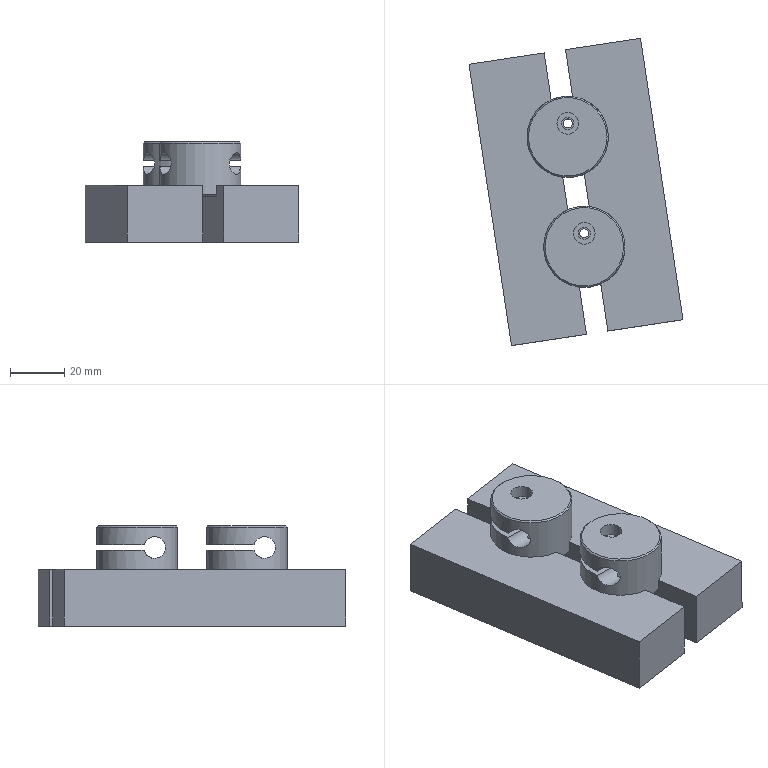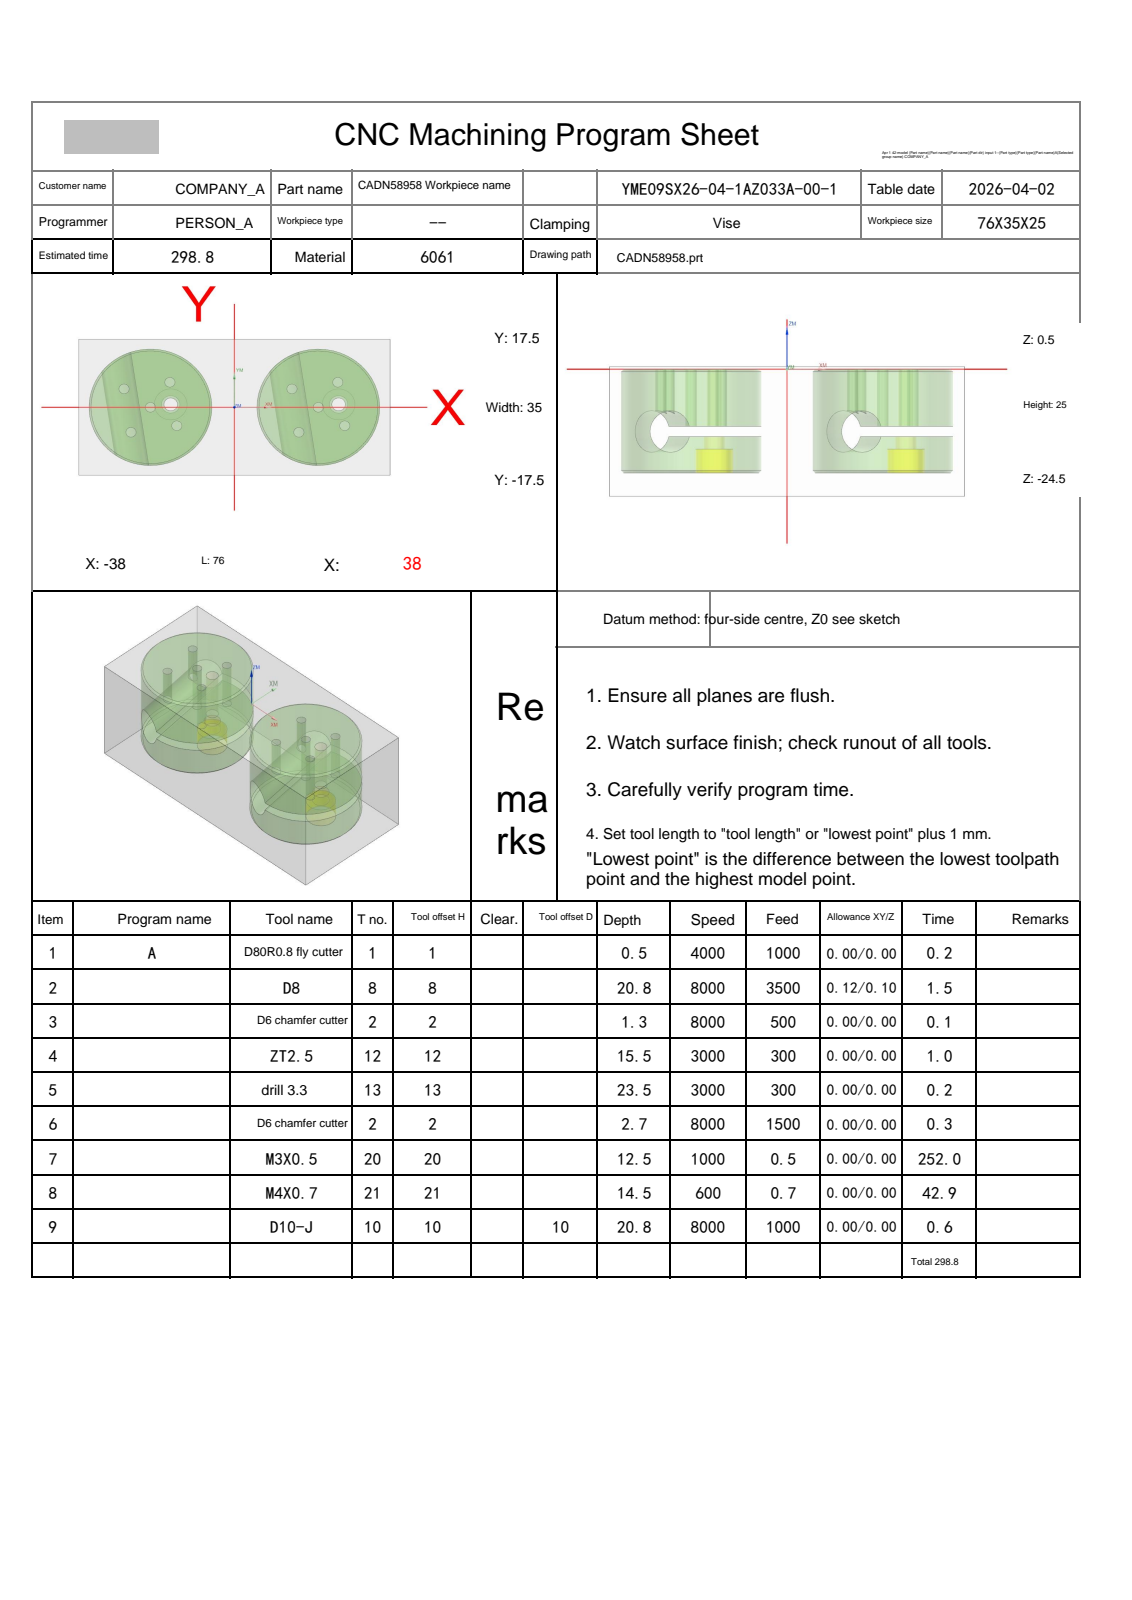NC program | NX | posted by the shop | part box 78.946 x 113.372 x 37 mm
Lines 35 to 955 of 2409:
N2 T08 M06
(D8  D=8. R=0. H=08 ce=0.12 di=0.10)
G00 G90 G54 X-19.131 Y27.067 M03 S8000
G43 H08 Z20.
M08
Z-8.15
G01 X-19.124 Y26.967 Z-8.775 F3500.
X-19.117 Y26.868 Z-9.022
X-19.11 Y26.768 Z-9.204
X-19.103 Y26.668 Z-9.35
X-19.096 Y26.568 Z-9.473
X-19.089 Y26.469 Z-9.578
X-19.082 Y26.369 Z-9.67
X-19.075 Y26.269 Z-9.75
X-19.068 Y26.169 Z-9.82
X-19.061 Y26.07 Z-9.882
X-19.054 Y25.97 Z-9.936
X-19.047 Y25.87 Z-9.983
X-19.04 Y25.77 Z-10.024
X-19.033 Y25.671 Z-10.058
X-19.026 Y25.571 Z-10.086
X-19.019 Y25.471 Z-10.11
X-19.012 Y25.371 Z-10.127
X-19.005 Y25.271 Z-10.14
X-18.998 Y25.172 Z-10.147
X-18.991 Y25.072 Z-10.15
X-18.87 Y23.364
G03 X-18.686 Y23.05 I.419 J.035
X-15.158 Y22.401 I3.636 J9.857
X-6.623 Y22.237 I8.535 J221.98
X-4.206 Y22.25 I0.0 J222.144
G01 X36.398 Y22.232
G02 X41.494 Y18.712 I-.081 J-5.567
X42.581 Y13.492 I-14.286 J-5.696
X42.772 Y3.965 I-236.709 J-9.527
X42.75 Y.694 I-236.9 J0.0
G01 X42.725 Y-16.025
G02 X39.097 Y-21.041 I-5.6 J.23
X33.548 Y-22.109 I-5.843 J15.421
X23.999 Y-22.267 I-9.549 J287.747
X20.83 Y-22.25 I0.0 J287.905
G01 X-36.393 Y-22.232
G02 X-41.526 Y-18.64 I.086 J5.587
X-42.591 Y-13.333 I14.752 J5.72
X-42.771 Y-3.796 I253.491 J9.537
X-42.75 Y-.536 I253.671 J0.0
X-42.773 Y5.952 I885.801 J6.487
X-42.715 Y16.169 I885.825 J0.0
X-39.185 Y21.006 I5.539 J-.335
X-33.883 Y22.088 I5.729 J-14.544
X-25.706 Y22.27 I8.177 J-183.855
X-20.686 Y22.201 I0.0 J-184.037
G03 X-9.011 Y21.46 I11.675 J91.591
X-8.195 Y21.464 I0.0 J92.332
G01 X34.811 Y21.426
G02 X40.2 Y17.823 I-.373 J-6.389
X41.681 Y12.131 I-13.504 J-6.553
X41.964 Y3.635 I-127.72 J-8.496
X41.947 Y1.578 I-128.003 J0.0
X41.973 Y-4.806 I-775.289 J-6.384
X41.913 Y-14.496 I-775.316 J0.0
X38.403 Y-19.658 I-6.387 J.569
X32.801 Y-21.164 I-6.537 J13.142
X24.513 Y-21.461 I-8.288 J115.221
X22.649 Y-21.446 I0.0 J115.519
G01 X-34.727 Y-21.43
G02 X-40.214 Y-17.796 I.294 J6.403
X-41.684 Y-12.101 I13.598 J6.547
X-41.963 Y-3.693 I126.62 J8.408
X-41.947 Y-1.708 I126.899 J0.0
X-41.972 Y4.733 I828.232 J6.441
X-41.915 Y14.482 I828.257 J0.0
X-38.313 Y19.705 I6.383 J-.547
X-32.7 Y21.174 I6.516 J-13.441
X-25.626 Y21.453 I7.074 J-89.522
X-20.709 Y21.319 I0.0 J-89.801
G03 X-6.747 Y20.649 I13.963 J145.3
X-5.413 Y20.655 I0.0 J145.97
G01 X33.146 Y20.625
G02 X39.263 Y16.567 I-.383 J-7.217
X40.827 Y10.73 I-14.356 J-6.973
X41.149 Y2.719 I-99.489 J-8.011
X41.142 Y1.539 I-99.811 J0.0
X41.163 Y-4.257 I-776.691 J-5.796
X41.117 Y-12.755 I-776.713 J0.0
X36.9 Y-18.848 I-7.25 J.512
X30.804 Y-20.369 I-7.073 J15.375
X21.958 Y-20.662 I-8.845 J133.127
X19.93 Y-20.647 I0.0 J133.42
G01 X-33.065 Y-20.629
G02 X-39.261 Y-16.568 I.308 J7.227
X-40.843 Y-10.573 I14.564 J7.048
X-41.164 Y-1.667 I123.489 J8.905
X-41.147 Y.38 I123.809 J0.0
X-41.166 Y5.016 I550.857 J4.636
X-41.11 Y12.859 I550.876 J0.0
X-37.08 Y18.757 I7.202 J-.597
X-31.244 Y20.325 I6.976 J-14.316
X-24.832 Y20.594 I6.412 J-76.248
X-17.332 Y20.226 I0.0 J-76.517
G03 X-4.66 Y19.845 I12.672 J210.701
X-2.952 Y19.852 I0.0 J211.082
G01 X31.485 Y19.828
G02 X38.478 Y15.184 I-.214 J-7.909
X40.047 Y8.852 I-16.47 J-7.442
X40.363 Y-.228 I-130.33 J-9.08
X40.346 Y-2.34 I-130.646 J0.0
X40.356 Y-5.181 I-401.006 J-2.84
X40.31 Y-11.253 I-401.016 J0.0
X35.685 Y-17.976 I-7.886 J.473
X29.274 Y-19.554 I-7.478 J16.576
X20.298 Y-19.859 I-8.975 J131.962
X18.4 Y-19.845 I0.0 J132.267
G01 X-31.481 Y-19.827
G02 X-38.529 Y-15.079 I.222 J7.934
X-40.065 Y-8.656 I16.993 J7.458
X-40.367 Y.785 I147.679 J9.442
X-40.35 Y3.017 I147.98 J0.0
X-40.37 Y5.925 I215.578 J2.908
X-40.3 Y11.403 I215.598 J0.0
X-35.678 Y17.981 I7.872 J-.618
X-29.266 Y19.555 I7.473 J-16.592
X-24.417 Y19.756 I4.85 J-58.435
X-19.996 Y19.589 I0.0 J-58.636
G03 X-2.9 Y19.035 I17.096 J263.295
X-.002 Y19.051 I0.0 J263.849
G01 X19.25
G02 X20.451 Y19.097 I1.202 J-15.465
X21.8 Y19.038 I0.0 J-15.511
X25.177 Y19.072 I3.378 J-171.509
X30.626 Y18.985 I0.0 J-171.543
X37.612 Y14.064 I-.668 J-8.367
X39.232 Y7.497 I-17.32 J-7.755
X39.594 Y-2.38 I-134.276 J-9.877
X39.558 Y-5.506 I-134.638 J0.0
X39.575 Y-6.817 I-50.379 J-1.311
X39.436 Y-10.557 I-50.396 J0.0
X34.526 Y-17.129 I-8.324 J1.099
X28.036 Y-18.728 I-7.725 J17.386
X22.263 Y-19.001 I-7.189 J90.654
X19.234 Y-19.112 I-3.029 J41.27
X17.453 Y-19.074 I0.0 J41.381
G01 X-19.382 Y-19.05
G02 X-20.679 Y-19.103 I-1.297 J15.704
X-21.703 Y-19.07 I0.0 J15.757
X-23.973 Y-19.08 I-2.27 J243.415
X-30.532 Y-18.992 I0.0 J243.425
X-37.642 Y-14.003 I.579 J8.385
X-39.223 Y-7.588 I17.344 J7.677
X-39.508 Y-1.583 I91.225 J7.339
X-39.608 Y.501 I21.702 J2.084
X-39.571 Y1.771 I21.802 J0.0
X-39.58 Y3.778 I221.12 J2.007
X-39.491 Y10.046 I221.129 J0.0
X-34.484 Y17.15 I8.389 J-.596
X-27.67 Y18.756 I7.796 J-17.815
X-23.917 Y18.883 I3.753 J-55.479
X-23.232 Y18.879 I0.0 J-55.606
G01 X-21.794 Y19.076
X-19.177 Y19.074
G03 X-9.127 Y18.324 I10.095 J67.538
X.407 Y18.251 I9.534 J623.015
G01 X.847
X14.941 Y18.256
X16.974 Y18.792
X19.721 Y19.104
X22.481 Y19.017
G03 X28.83 Y18.277 I7.157 J33.779
G02 X36.914 Y12.671 I-.276 J-9.029
X38.388 Y6.63 I-18.905 J-7.815
X39.511 Y1.852 I-15.348 J-6.128
G03 X37.94 Y7.743 I-17.822 J-1.597
X36.288 Y12.186 I-35.429 J-10.649
X29.471 Y17.247 I-8.285 J-4.036
G01 X28.174 Y17.485
X27.822 Y17.662
X25.043 Y18.561
X27.822 Y17.662
G02 X32.016 Y15.391 I-14.292 J-31.391
X34.191 Y13.303 I-6.362 J-8.805
G01 X34.568 Y12.949
X36.287 Y10.787
X37.676 Y8.4
X37.945 Y7.732
X37.676 Y8.4
X36.287 Y10.787
X34.568 Y12.949
X32.555 Y14.841
X30.291 Y16.423
G02 X30.12 Y16.74 I.24 J.334
G01 X30.108 Y17.16
X30.065 Y18.731 Z-10.05
X30.043 Y19.549
X30.036 Y19.611
X30.02 Y19.67
X29.996 Y19.727
X29.962 Y19.779
X29.921 Y19.825
X29.874 Y19.865
X29.821 Y19.897
X29.763 Y19.92
X28.826 Y20.215
X28.451 Y20.329
X28.073 Y20.435
X27.693 Y20.533
X27.31 Y20.622
X26.926 Y20.702
X24.991 Y21.087
X24.468 Y21.185
X23.943 Y21.274
X23.417 Y21.352
X22.889 Y21.419
X22.36 Y21.477
X21.83 Y21.524
X21.299 Y21.561
X20.767 Y21.587
X20.235 Y21.603
X19.703 Y21.609
X19.171 Y21.604
X16.233 Y21.548
X16.167 Y21.542
X16.103 Y21.524
X16.043 Y21.496
X15.989 Y21.459
X15.941 Y21.413
X15.901 Y21.36
X15.871 Y21.302
X15.851 Y21.239
X15.681 Y20.503
X15.326 Y18.972 Z-10.15
X15.268 Y18.702
G02 X14.941 Y18.256 I-.51 J.031
X10.406 Y17.673 I-4.535 J17.342
X10.165 Y17.675 I0.0 J17.925
X1.423 Y17.589 I-8.742 J446.105
X-12.604 Y17.809 I0.0 J446.191
G01 X-13.803 Y17.89
G03 X-16.584 Y18.715 I-10.094 J-28.945
G02 X-13.803 Y17.89 I-7.313 J-29.769
G03 X-10.357 Y17.091 I3.876 J8.891
X-1.36 Y16.799 I8.998 J138.056
X.661 Y16.813 I0.0 J138.349
X3.503 Y16.789 I2.842 J165.087
X11.675 Y16.991 I0.0 J165.112
G01 X14.305 Y18.088
G02 X11.006 Y16.714 I-21.045 J45.858
X6.202 Y16.226 I-4.804 J23.407
X5.95 Y16.227 I0.0 J23.895
X.579 Y16.153 I-5.371 J195.779
X-9.312 Y16.403 I0.0 J195.853
X-11.138 Y16.634 I3.588 J35.774
G03 X-13.279 Y17.661 I-6.716 J-11.25
G02 X-10.585 Y16.33 I-6.774 J-17.104
G03 X-6.194 Y15.558 I4.692 J13.802
X.794 Y15.365 I6.989 J126.47
X8.309 Y15.588 I0.0 J126.663
G01 X9.775 Y15.797
X11.757 Y17.003
G02 X9.24 Y15.524 I-15.23 J23.032
X4.937 Y14.863 I-4.434 J14.537
X.3 Y14.746 I-4.636 J91.433
X-7.316 Y15.063 I0.0 J91.55
X-9.228 Y15.423 I.857 J9.806
G03 X-10.867 Y16.468 I-11.198 J-15.762
G02 X-8.749 Y15.098 I-18.982 J-31.674
G03 X-4.759 Y14.207 I4.509 J10.809
X.568 Y13.977 I5.327 J61.562
X6.809 Y14.293 I0.0 J61.792
X8.232 Y14.601 I-1.459 J10.189
G02 X9.609 Y15.695 I13.192 J-15.177
G03 X7.939 Y14.398 I59.431 J-78.222
G02 X4.35 Y13.565 I-4.004 J9.097
X.202 Y13.38 I-4.148 J46.446
X-6.183 Y13.819 I0.0 J46.631
X-7.767 Y14.228 I2.736 J13.873
G01 X-9.067 Y15.292
G03 X-7.103 Y13.773 I10.362 J11.366
X-2.789 Y12.806 I4.821 J11.403
X.481 Y12.646 I3.27 J33.308
X5.893 Y13.086 I0.0 J33.468
X6.907 Y13.404 I-.579 J3.627
G02 X8.2 Y14.575 I5.94 J-5.263
G03 X6.795 Y13.291 I5.268 J-7.181
G02 X3.736 Y12.324 I-3.595 J6.05
X.145 Y12.09 I-3.591 J27.415
X-5.206 Y12.612 I0.0 J27.649
X-6.651 Y13.118 I1.286 J5.986
G01 X-7.532 Y14.036
G03 X-6.226 Y12.735 I12.896 J11.636
X-2.596 Y11.607 I4.333 J7.543
X.382 Y11.397 I2.979 J20.969
X4.946 Y11.894 I0.0 J21.179
X5.845 Y12.236 I-.923 J3.783
G01 X6.868 Y13.361
G02 X5.58 Y11.999 I-14.64 J12.555
X2.237 Y11.006 I-3.789 J6.634
X.079 Y10.871 I-2.158 J17.112
X-4.809 Y11.578 I0.0 J17.247
X-5.628 Y12.016 I.325 J1.59
G01 X-6.498 Y12.954
X-5.26 Y11.602
G03 X-1.78 Y10.396 I4.096 J6.196
X.351 Y10.227 I2.131 J13.405
X4.505 Y10.879 I0.0 J13.573
X5.025 Y11.162 I-.687 J1.881
G02 X5.826 Y12.215 I6.252 J-3.923
G03 X4.929 Y11.035 I6.647 J-5.979
G02 X2.149 Y9.928 I-3.299 J4.241
X.077 Y9.746 I-2.073 J11.7
X-4.318 Y10.588 I0.0 J11.882
G01 X-4.843 Y10.896
X-5.531 Y11.879
G03 X-4.375 Y10.404 I5.918 J3.45
X-.57 Y9.214 I4.027 J6.201
X.431 Y9.159 I1. J8.988
X4.159 Y9.963 I0.0 J9.044
X4.992 Y11.113 I-5.911 J5.159
G02 X4.034 Y9.799 I-6.491 J3.729
X.706 Y8.759 I-3.378 J4.963
X-.038 Y8.727 I-.744 J8.484
X-3.958 Y9.683 I0.0 J8.517
X-4.769 Y10.79 I7.943 J6.665
G03 X-3.79 Y9.429 I9.764 J5.993
X-.289 Y8.221 I3.59 J4.725
X.403 Y8.185 I.692 J6.721
X3.64 Y9.011 I0.0 J6.757
G01 X4.24 Y10.015
G03 X3.649 Y8.975 I9.638 J-6.168
G02 X1.08 Y7.869 I-2.89 J3.18
X.015 Y7.784 I-1.064 J6.602
X-3.51 Y8.789 I0.0 J6.687
X-4.078 Y9.779 I3.073 J2.421
G03 X-3.23 Y8.402 I4.119 J1.589
X.119 Y7.291 I3.349 J4.491
X.817 Y7.335 I0.0 J5.602
X3.203 Y8.108 I-.262 J4.875
G01 X3.698 Y9.049
G02 X3.073 Y7.92 I-4.147 J1.557
X.224 Y6.932 I-2.849 J3.61
X-.19 Y6.95 I0.0 J4.599
X-3.094 Y7.899 I.055 J5.09
G01 X-3.581 Y8.811
G03 X-2.851 Y7.552 I4.907 J2.003
X.123 Y6.478 I2.975 J3.583
X.831 Y6.532 I0.0 J4.657
X2.77 Y7.224 I-.312 J3.933
G01 X3.268 Y8.186
G02 X2.652 Y7.043 I-5.442 J2.193
X.097 Y6.146 I-2.556 J3.192
X-.641 Y6.213 I0.0 J4.089
X-2.771 Y7.128 I.287 J3.606
G01 X-3.077 Y7.828
X-2.655 Y6.895
G03 X-.002 Y5.752 I2.652 J2.507
G01 X.195 Y5.757
X.306 Y5.756
G03 X2.513 Y6.481 I0.0 J3.721
X2.839 Y7.326 I-3.327 J1.769
G02 X2.423 Y6.317 I-2.914 J.613
X.059 Y5.432 I-2.364 J2.711
X-.798 Y5.535 I0.0 J3.597
X-2.49 Y6.357 I.585 J3.358
G01 X-2.785 Y7.127
G03 X-2.165 Y5.892 I2.618 J.541
X.14 Y5.065 I2.305 J2.799
X2.275 Y5.76 I0.0 J3.626
X2.581 Y6.558 I-4.48 J2.177
G02 X2.168 Y5.581 I-2.62 J.532
X-.004 Y4.775 I-2.172 J2.523
X-1.381 Y5.073 I0.0 J3.329
X-2.291 Y5.718 I.717 J1.978
G01 X-2.529 Y6.397
G03 X-1.917 Y5.174 I2.581 J.528
X.128 Y4.44 I2.045 J2.481
X2.042 Y5.072 I0.0 J3.215
X2.351 Y5.874 I-3.801 J1.927
G02 X1.943 Y4.901 I-2.661 J.545
X.005 Y4.177 I-1.939 J2.232
X-2.018 Y4.977 I0.0 J2.956
G01 X-2.277 Y5.678
G03 X-1.809 Y4.623 I2.713 J.572
X.117 Y3.858 I1.926 J2.044
X1.885 Y4.486 I0.0 J2.808
G01 X2.102 Y5.132
X1.924 Y4.493
G02 X.109 Y3.619 I-1.815 J1.446
X-.285 Y3.652 I0.0 J2.32
X-1.914 Y4.454 I.165 J2.393
G01 X-2.054 Y5.017
G03 X-.766 Y3.478 I1.675 J.093
X.111 Y3.321 I.878 J2.371
X1.794 Y3.963 I0.0 J2.528
X1.952 Y4.573 I-2.799 J1.048
G02 X.945 Y3.276 I-1.343 J.003
X.025 Y3.098 I-.92 J2.298
X-1.798 Y3.898 I0.0 J2.476
G01 X-1.955 Y4.541
G03 X-.48 Y2.895 I1.729 J.065
X.112 Y2.82 I.591 J2.29
X1.681 Y3.416 I0.0 J2.365
X1.868 Y4.131 I-2.003 J.906
G02 X1.62 Y3.276 I-1.842 J.072
X.007 Y2.607 I-1.613 J1.611
X-1.686 Y3.361 I0.0 J2.279
G01 X-1.826 Y3.924
G03 X-.3 Y2.384 I1.64 J.099
X.134 Y2.338 I.434 J2.053
X1.613 Y2.948 I0.0 J2.099
G01 X1.756 Y3.535
Y3.531
G02 X.701 Y2.249 I-1.306 J0.0
X.023 Y2.141 I-.679 J2.078
X-1.567 Y2.827 I0.0 J2.186
G01 X-1.718 Y3.406
G03 X-.346 Y1.938 I1.54 J.065
X.119 Y1.883 I.465 J1.944
X1.512 Y2.449 I0.0 J1.999
X1.68 Y3.129 I-3.67 J1.263
G02 X1.423 Y2.275 I-1.768 J.065
X.016 Y1.7 I-1.407 J1.434
X-1.511 Y2.403 I0.0 J2.009
G01 X-1.606 Y2.871
Y2.869
G03 X-.532 Y1.555 I1.34 J0.0
X.09 Y1.455 I.622 J1.873
X1.425 Y1.975 I0.0 J1.974
X1.586 Y2.632 I-3.815 J1.283
G02 X1.381 Y1.861 I-1.683 J.033
X.013 Y1.262 I-1.369 J1.267
X-1.499 Y2.035 I0.0 J1.865
G01 X-1.559 Y2.53
X-1.564 Y2.418
G03 X-.525 Y1.139 I1.306 J0.0
X.091 Y1.029 I.616 J1.658
X1.444 Y1.658 I0.0 J1.769
X1.51 Y2.198 I-3.756 J.732
G01 X1.524 Y2.026
G02 X.767 Y1.02 I-1.047 J0.0
X.02 Y.862 I-.747 J1.694
X-1.456 Y1.596 I0.0 J1.852
G01 X-1.525 Y2.108
X-1.53 Y1.998
G03 X-.467 Y.72 I1.3 J0.0
X.101 Y.621 I.568 J1.581
X1.435 Y1.28 I0.0 J1.68
G01 X1.494 Y1.876
X1.505 Y1.705
G02 X1.35 Y1.072 I-1.368 J0.0
X.006 Y.468 I-1.344 J1.19
X-1.412 Y1.163 I0.0 J1.795
X-1.493 Y1.697 I4.63 J.972
G01 X-1.498 Y1.584
G03 X-.415 Y.313 I1.287 J0.0
X.081 Y.241 I.495 J1.681
X1.393 Y.832 I0.0 J1.753
X1.471 Y1.399 I-2.014 J.567
G01 Y1.404
X1.482 Y1.251
G02 X.588 Y.168 I-1.103 J0.0
X.013 Y.07 I-.576 J1.645
X-1.391 Y.78 I0.0 J1.743
G01 X-1.454 Y1.213
X-1.456 Y1.152
G03 X-.387 Y-.083 I1.248 J0.0
X.082 Y-.148 I.47 J1.657
X1.374 Y.435 I0.0 J1.722
X1.448 Y.928 I-2.106 J.57
G01 X1.456 Y.802
G02 X.736 Y-.163 I-1.006 J0.0
X.018 Y-.322 I-.719 J1.538
X-1.367 Y.394 I0.0 J1.697
G01 X-1.429 Y.891
X-1.434 Y.772
G03 X-.325 Y-.477 I1.257 J0.0
X.125 Y-.544 I.45 J1.468
X1.384 Y.112 I0.0 J1.536
G01 X1.429 Y.536
X1.436 Y.417
G02 X.664 Y-.57 I-1.016 J0.0
X.018 Y-.701 I-.646 J1.519
X-1.359 Y.039 I0.0 J1.651
G01 X-1.395 Y.472
X-1.406 Y.318
G03 X-.532 Y-.793 I1.144 J0.0
X.09 Y-.919 I.622 J1.479
X1.356 Y-.299 I0.0 J1.604
G01 X1.41 Y.144
X1.417 Y.027
G02 X.665 Y-.943 I-1. J0.0
X.026 Y-1.068 I-.639 J1.558
X-1.366 Y-.332 I0.0 J1.684
X-1.392 Y.05 I2.81 J.383
G01 X-1.39 Y.16
G03 X-1.413 Y-.066 I1.094 J-.227
X-.61 Y-1.139 I1.117 J0.0
X.07 Y-1.282 I.68 J1.536
X1.33 Y-.713 I0.0 J1.68
X1.396 Y-.154 I-2.367 J.562
G01 X1.408 Y-.324
G02 X1.309 Y-.807 I-1.229 J0.0
X.014 Y-1.45 I-1.294 J.982
X-1.401 Y-.623 I0.0 J1.625
G01 X-1.406 Y-.194
G03 X-1.429 Y-.422 I1.112 J-.227
X-.623 Y-1.508 I1.135 J0.0
X.066 Y-1.656 I.689 J1.527
X1.363 Y-1.041 I0.0 J1.676
X1.414 Y-.709 I-1.066 J.332
X1.393 Y-.497 I-1.117 J0.0
G02 X1.427 Y-.746 I-.909 J-.249
X.781 Y-1.64 I-.942 J0.0
X.023 Y-1.817 I-.757 J1.535
X-1.398 Y-1.06 I0.0 J1.712
X-1.427 Y-.688 I2.342 J.371
G01 X-1.424 Y-.564
G03 X-1.446 Y-.791 I1.121 J-.227
X-.632 Y-1.886 I1.143 J0.0
X.064 Y-2.036 I.696 J1.534
X1.408 Y-1.368 I0.0 J1.685
X1.445 Y-1.044 I-1.396 J.323
X1.418 Y-.77 I-1.433 J0.0
G02 X1.465 Y-1.073 I-.949 J-.303
X.804 Y-2.011 I-.996 J0.0
X.023 Y-2.198 I-.781 J1.536
X-1.42 Y-1.417 I0.0 J1.723
X-1.441 Y-.996 I4.174 J.421
G01 Y-.929
G03 X-1.465 Y-1.161 I1.124 J-.233
X-.672 Y-2.253 I1.148 J0.0
X.065 Y-2.42 I.737 J1.536
X1.441 Y-1.721 I0.0 J1.703
X1.476 Y-1.402 I-1.453 J.319
X1.45 Y-1.126 I-1.487 J0.0
G02 X1.498 Y-1.433 I-.966 J-.307
X.836 Y-2.384 I-1.014 J0.0
X.025 Y-2.584 I-.811 J1.543
X-1.436 Y-1.793 I0.0 J1.743
X-1.46 Y-1.399 I3.214 J.393
G01 X-1.458 Y-1.302
G03 X-1.481 Y-1.532 I1.143 J-.23
X-.661 Y-2.645 I1.165 J0.0
X.077 Y-2.815 I.738 J1.513
X1.491 Y-2.046 I0.0 J1.683
X1.499 Y-1.816 I-3.181 J.23
X1.483 Y-1.496 I-3.189 J0.0
G02 X1.524 Y-1.791 I-1.031 J-.295
X.725 Y-2.828 I-1.073 J0.0
X.019 Y-2.979 I-.706 J1.578
X-1.468 Y-2.131 I0.0 J1.728
G01 X-1.477 Y-1.694
G03 X-1.498 Y-1.918 I1.142 J-.224
X-.697 Y-3.024 I1.164 J0.0
X.083 Y-3.212 I.779 J1.518
X1.527 Y-2.414 I0.0 J1.706
G01 X1.531 Y-2.235
G03 X1.517 Y-1.873 I-4.791 J0.0
G02 X1.558 Y-2.168 I-1.046 J-.295
X.757 Y-3.217 I-1.087 J0.0
X.027 Y-3.374 I-.73 J1.612
X-1.499 Y-2.501 I0.0 J1.769
G01 X-1.512 Y-2.309
G02 X-1.495 Y-2.096 I1.358 J0.0
G03 X-1.531 Y-2.364 I.987 J-.269
X-.966 Y-3.279 I1.023 J0.0
X.073 Y-3.601 I1.039 J1.513
X1.542 Y-2.866 I0.0 J1.835
X1.579 Y-2.541 I-1.38 J.325
X1.552 Y-2.267 I-1.418 J0.0
G02 X1.599 Y-2.575 I-.988 J-.308
X.973 Y-3.527 I-1.035 J0.0
X.041 Y-3.78 I-.931 J1.588
X-1.561 Y-2.844 I0.0 J1.841
X-1.579 Y-2.637 I1.202 J.207
X-1.536 Y-2.315 I1.22 J0.0
G03 X-1.598 Y-2.686 I1.08 J-.371
X-.933 Y-3.723 I1.142 J0.0
X.072 Y-4.021 I1.004 J1.545
X1.588 Y-3.225 I0.0 J1.843
X1.603 Y-2.942 I-2.777 J.283
X1.584 Y-2.62 I-2.791 J0.0
G02 X1.627 Y-2.931 I-1.102 J-.311
X.805 Y-4.03 I-1.145 J0.0
X.029 Y-4.197 I-.776 J1.716
X-1.645 Y-3.177 I0.0 J1.883
G01 Y-3.139
G02 X-1.603 Y-2.684 I2.494 J0.0
G03 X-1.667 Y-3.062 I1.104 J-.378
X-1.037 Y-4.098 I1.167 J0.0
X.06 Y-4.44 I1.097 J1.589
X1.645 Y-3.61 I0.0 J1.931
X1.682 Y-3.352 I-.888 J.259
X1.62 Y-3.018 I-.925 J0.0
G02 X1.697 Y-3.397 I-.893 J-.379
X1.194 Y-4.247 I-.97 J0.0
X.031 Y-4.628 I-1.163 J1.585
X-1.717 Y-3.563 I0.0 J1.966
G01 Y-3.54
G02 X-1.674 Y-3.07 I2.643 J0.0
G03 X-1.737 Y-3.452 I1.142 J-.382
X-1.076 Y-4.526 I1.204 J0.0
X.059 Y-4.879 I1.135 J1.648
X1.746 Y-3.955 I0.0 J2.002
X1.767 Y-3.734 I-1.156 J.221
X1.687 Y-3.309 I-1.177 J0.0
G02 X1.789 Y-3.756 I-.932 J-.447
X1.294 Y-4.638 I-1.034 J0.0
X.03 Y-5.076 I-1.263 J1.605
X-1.79 Y-3.96 I0.0 J2.042
G01 Y-3.913
G02 X-1.733 Y-3.389 I2.439 J0.0
G03 X-1.809 Y-3.829 I1.23 J-.44
X-1.029 Y-5.025 I1.307 J0.0
X.063 Y-5.333 I1.093 J1.781
X1.834 Y-4.354 I0.0 J2.089
X1.858 Y-4.12 I-1.106 J.233
X1.778 Y-3.703 I-1.131 J0.0
G02 X1.874 Y-4.153 I-1.016 J-.451
X1.28 Y-5.137 I-1.112 J0.0
X.034 Y-5.532 I-1.246 J1.769
X-1.848 Y-4.436 I0.0 J2.164
X-1.872 Y-4.196 I1.203 J.24
X-1.812 Y-3.817 I1.227 J0.0
G03 X-1.884 Y-4.25 I1.252 J-.432
X-1.154 Y-5.434 I1.325 J0.0
X.069 Y-5.805 I1.223 J1.825
X1.933 Y-4.77 I0.0 J2.197
X1.955 Y-4.545 I-1.14 J.225
X1.875 Y-4.122 I-1.162 J0.0
G02 X1.978 Y-4.58 I-.976 J-.458
X1.52 Y-5.462 I-1.078 J0.0
X.041 Y-6.014 I-1.479 J1.703
X-1.916 Y-4.88 I0.0 J2.255
X-1.949 Y-4.604 I1.134 J.276
X-1.888 Y-4.23 I1.167 J0.0
G03 X-1.966 Y-4.683 I1.27 J-.453
X-1.274 Y-5.861 I1.349 J0.0
X.075 Y-6.298 I1.349 J1.863
X2.023 Y-5.22 I0.0 J2.3
X2.057 Y-4.959 I-1.008 J.261
X1.976 Y-4.557 I-1.042 J0.0
G02 X2.065 Y-5.008 I-1.101 J-.451
X1.468 Y-6.04 I-1.19 J0.0
X.049 Y-6.522 I-1.42 J1.845
X-2.041 Y-5.221 I0.0 J2.328
G01 X-2.042 Y-5.155
G02 X-1.963 Y-4.642 I1.719 J0.0
G03 X-2.065 Y-5.146 I1.193 J-.504
X-1.545 Y-6.183 I1.295 J0.0
X.077 Y-6.807 I1.622 J1.799
X2.108 Y-5.704 I0.0 J2.422
X2.155 Y-5.377 I-1.118 J.327
X2.059 Y-4.915 I-1.164 J0.0
G02 X2.172 Y-5.435 I-1.147 J-.521
X1.585 Y-6.5 I-1.259 J0.0
X.05 Y-7.03 I-1.535 J1.956
X-2.071 Y-5.841 I0.0 J2.487
X-2.182 Y-5.423 I.727 J.418
X-2.05 Y-4.971 I.839 J0.0
G03 X-2.2 Y-5.584 I1.177 J-.613
X-1.69 Y-6.631 I1.327 J0.0
X.076 Y-7.333 I1.766 J1.869
X2.167 Y-6.259 I0.0 J2.572
X2.291 Y-5.886 I-.502 J.373
X2.214 Y-5.586 I-.625 J0.0
G01 X2.178 Y-5.43
G02 X2.306 Y-6.026 I-1.329 J-.596
G01 X2.304 Y-6.09
G02 X.23 Y-7.55 I-2.074 J.744
G01 X.203 Y-7.549
G02 X-.048 Y-7.562 I-.251 J2.422
X-2.315 Y-6.017 I0.0 J2.435
G01 X-2.318 Y-5.934
G02 X-2.19 Y-5.384 I1.246 J0.0
G03 X-2.346 Y-6.028 I1.25 J-.644
X-1.795 Y-7.144 I1.406 J0.0
X.075 Y-7.884 I1.87 J1.993
X2.287 Y-6.756 I0.0 J2.733
X2.443 Y-6.264 I-.703 J.492
G01 X2.437 Y-6.169
X2.266 Y-5.72
G02 X2.458 Y-6.38 I-1.038 J-.66
X2.03 Y-7.313 I-1.23 J0.0
X.052 Y-8.134 I-1.978 J1.97
X-2.367 Y-6.735 I0.0 J2.791
X-2.464 Y-6.298 I.939 J.438
X-2.32 Y-5.771 I1.036 J0.0
G03 X-2.5 Y-6.483 I1.325 J-.713
X-1.92 Y-7.67 I1.505 J0.0
X.079 Y-8.459 I1.999 J2.138
X2.399 Y-7.316 I0.0 J2.927
X2.604 Y-6.716 I-.777 J.6
X2.437 Y-6.169 I-.982 J0.0
G02 X2.633 Y-6.848 I-1.081 J-.679
X2.219 Y-7.789 I-1.277 J0.0
X.051 Y-8.717 I-2.168 J2.068
X-2.465 Y-7.347 I0.0 J2.996
X-2.626 Y-6.784 I.901 J.563
X-2.482 Y-6.249 I1.063 J0.0
G03 X-2.661 Y-6.974 I1.382 J-.725
X-2.07 Y-8.196 I1.56 J0.0
X.084 Y-9.065 I2.154 J2.236
X2.591 Y-7.791 I0.0 J3.105
X2.787 Y-7.2 I-.793 J.591
X2.623 Y-6.654 I-.989 J0.0
G02 X2.82 Y-7.341 I-1.099 J-.688
X2.441 Y-8.257 I-1.296 J0.0
X.053 Y-9.333 I-2.388 J2.113
X-2.611 Y-7.896 I0.0 J3.189
X-2.796 Y-7.291 I.896 J.604
X-2.651 Y-6.751 I1.08 J0.0
G03 X-2.832 Y-7.491 I1.424 J-.74
X-2.274 Y-8.707 I1.605 J0.0
X.088 Y-9.696 I2.362 J2.327
X2.782 Y-8.314 I0.0 J3.316
X2.988 Y-7.699 I-.814 J.615
G01 X2.983 Y-7.594
X2.783 Y-7.071
G02 X3.02 Y-7.943 I-1.572 J-.895
X.959 Y-9.847 I-2.536 J.678
X.031 Y-9.979 I-.928 J3.199
X-2.795 Y-8.411 I0.0 J3.331
X-2.978 Y-7.812 I.891 J.599
X-2.821 Y-7.252 I1.074 J0.0
G03 X-3.043 Y-8.076 I1.416 J-.824
G01 X-3.042 Y-8.105
G03 X-1.051 Y-10.149 I2.675 J.613
X.121 Y-10.353 I1.173 J3.278
X2.99 Y-8.844 I0.0 J3.481
X3.188 Y-8.285 I-.689 J.559
X3.156 Y-8.047 I-.887 J0.0
G01 X2.984 Y-7.598
G02 X3.234 Y-8.407 I-1.621 J-.944
X1.431 Y-10.379 I-2.561 J.532
X.063 Y-10.645 I-1.367 J3.381
X-2.917 Y-9.1 I0.0 J3.647
X-3.205 Y-8.225 I1.184 J.875
G01 X-3.193 Y-8.038
X-2.976 Y-7.61
G03 X-3.277 Y-8.526 I1.249 J-.917
X-2.938 Y-9.493 I1.55 J0.0
X.107 Y-11.039 I3.045 J2.225
X3.163 Y-9.477 I0.0 J3.771
X3.424 Y-8.728 I-.943 J.749
X3.401 Y-8.492 I-1.204 J0.0
G01 X3.17 Y-8.072
G02 X3.476 Y-8.92 I-1.023 J-.849
X3.212 Y-9.715 I-1.33 J0.0
X.092 Y-11.348 I-3.12 J2.166
X-1.126 Y-11.147 I0.0 J3.798
X-3.437 Y-8.934 I.768 J3.116
G01 X-3.45 Y-8.766
G02 X-3.215 Y-8.079 I1.117 J0.0
G03 X-3.525 Y-9.053 I1.372 J-.974
X-3.145 Y-10.119 I1.682 J0.0
X.114 Y-11.751 I3.259 J2.436
X3.337 Y-10.166 I0.0 J4.068
X3.693 Y-9.202 I-1.128 J.964
X3.678 Y-8.995 I-1.484 J0.0
G01 X3.408 Y-8.505
G02 X3.76 Y-9.32 I-1.507 J-1.133
X2.273 Y-11.477 I-2.759 J.311
X.083 Y-12.096 I-2.19 J3.565
X-3.433 Y-10.182 I0.0 J4.184
X-3.715 Y-9.246 I1.41 J.936
X-3.703 Y-9.041 I1.692 J0.0
G01 X-3.449 Y-8.542
G03 X-3.797 Y-9.595 I1.422 J-1.054
X-3.436 Y-10.667 I1.77 J0.0
G02 X-2.684 Y-11.708 I-7.261 J-6.035
X-2.495 Y-12.843 I-3.306 J-1.134
X-3.315 Y-15.093 I-3.495 J0.0
X-7.265 Y-17.516 I-5.505 J4.541
X-13.351 Y-18.194 I-6.087 J27.005
X-13.614 Y-18.193 I0.0 J27.683
G01 X-14.687 Y-18.213
X-17.342 Y-18.857
X-19.413 Y-19.052
X-17.342 Y-18.857
G03 X-13.519 Y-17.87 I-20.45 J87.05
X-8.947 Y-17.149 I-29.748 J203.73
X-6.533 Y-16.155 I-.728 J5.195
X-4.799 Y-12.558 I-3.987 J4.139
G02 X-4.5 Y-10.401 I25.456 J-2.429
G03 X-3.717 Y-9.07 I-5.426 J4.087
G02 X-4.669 Y-10.661 I-8.325 J3.901
X-5.593 Y-12.759 I-42.799 J17.595
X-9.57 Y-15.848 I-6.367 J4.093
G01 X-10.215 Y-16.081
X-12.12 Y-17.185
X-14.421 Y-18.109
X-12.12 Y-17.185
X-9.742 Y-15.806
X-7.587 Y-14.1
X-5.698 Y-12.103
X-4.547 Y-10.467
G02 X-4.267 Y-10.287 I.377 J-.278
G01 X-3.446 Y-10.129
X-1.903 Y-9.832 Z-10.05
X1.531 Y-9.173
X3.074 Y-8.876 Z-10.15
G02 X3.293 Y-8.84 I.219 J-.638
X3.516 Y-8.878 I0.0 J-.674
X3.853 Y-9.595 I-.598 J-.718
X3.781 Y-9.954 I-.934 J0.0
X2.821 Y-11.454 I-3.31 J1.06
G03 X2.372 Y-13.095 I2.774 J-1.641
X2.861 Y-14.802 I3.223 J0.0
X6.538 Y-17.578 I5.339 J3.247
X12.128 Y-18.339 I5.59 J20.158
G01 X12.152
X15.462 Y-18.409
X17.521 Y-18.886
X20.238 Y-19.118
X17.521 Y-18.886
G02 X13.478 Y-17.903 I84.925 J357.793
X8.712 Y-17.17 I11.786 J92.5
X5.475 Y-14.405 I.601 J3.982
X4.81 Y-10.964 I14.264 J4.539
G03 X4.427 Y-10.355 I-1.715 J-.655
G01 X3.732 Y-9.094
G03 X4.924 Y-11.08 I17.092 J8.906
X5.868 Y-13.287 I16.614 J5.798
X9.85 Y-16.227 I6.113 J4.113
G01 X11.18 Y-16.639
X12.323 Y-17.283
X14.709 Y-18.21
X12.323 Y-17.283
X9.948 Y-15.944
X7.855 Y-14.342
X6.004 Y-12.467
X4.759 Y-10.8
G03 X4.439 Y-10.64 I-.32 J-.239
X4.039 Y-11.04 I0.0 J-.4
G01 X4.04 Y-11.067
X4.086 Y-11.743
X4.194 Y-13.311 Z-10.05
X4.245 Y-14.057
X4.253 Y-14.114
X4.27 Y-14.17
X4.294 Y-14.222
X4.325 Y-14.271
X4.364 Y-14.314
X6.464 Y-16.382
X6.7 Y-16.608
X6.942 Y-16.827
X7.191 Y-17.039
X7.445 Y-17.244
X7.705 Y-17.441
X7.971 Y-17.631
X8.296 Y-17.851
X8.627 Y-18.061
X8.964 Y-18.262
X9.306 Y-18.454
X9.653 Y-18.636
X11.406 Y-19.525
X11.758 Y-19.697
X12.115 Y-19.859
X12.477 Y-20.01
X12.843 Y-20.151
X13.213 Y-20.282
X13.586 Y-20.402
X13.963 Y-20.514
X14.342 Y-20.616
X14.723 Y-20.71
X15.106 Y-20.794
X20.163 Y-21.847
X20.226 Y-21.855
X20.29 Y-21.853
X20.352 Y-21.84
X20.412 Y-21.818
X20.468 Y-21.787
X20.518 Y-21.748
X20.56 Y-21.701
X20.595 Y-21.648
X20.912 Y-21.072
X21.668 Y-19.694 Z-10.15
X21.973 Y-19.152
G02 X22.263 Y-19.001 I.323 J-.266
G01 X22.96 Y-18.961
G02 X29.28 Y-17.912 I16.829 J-81.816
G03 X34.953 Y-15.859 I-1.886 J14.08
X38.46 Y-10.113 I-4.924 J6.949
X38.873 Y-5.191 I-33.732 J5.307
X39.604 Y-.771 I-19.387 J5.479
G02 X38.406 Y-6.722 I-21.673 J1.266
X37.333 Y-10.813 I-33.572 J6.624
X32.05 Y-15.991 I-8.577 J3.467
X29.459 Y-16.836 I-8.632 J22.074
G01 X28.2 Y-17.501
X25.632 Y-18.418
X25.005 Y-18.546
X25.632 Y-18.418
X28.2 Y-17.501
G03 X33.381 Y-14.45 I-16.022 J33.135
X36.285 Y-10.76 I-6.05 J7.75
X37.777 Y-8.19 I-30.859 J19.627
G01 X38.619 Y-6.028
X37.777 Y-8.19
G02 X36.285 Y-10.76 I-32.351 J17.057
G01 X34.772 Y-12.724
X32.817 Y-14.624
X30.611 Y-16.228
G03 X30.446 Y-16.556 I.244 J-.328
G01 Y-16.562
X30.456 Y-16.934
X30.498 Y-18.505 Z-10.05
X30.52 Y-19.343
X30.516 Y-19.41
X30.501 Y-19.476
X30.474 Y-19.539
X30.438 Y-19.596
X30.393 Y-19.646
X30.339 Y-19.688
X30.28 Y-19.72
X30.215 Y-19.742
X25.446 Y-20.913
X25.063 Y-21.002
X24.679 Y-21.082
X24.293 Y-21.153
X23.906 Y-21.215
X23.517 Y-21.268